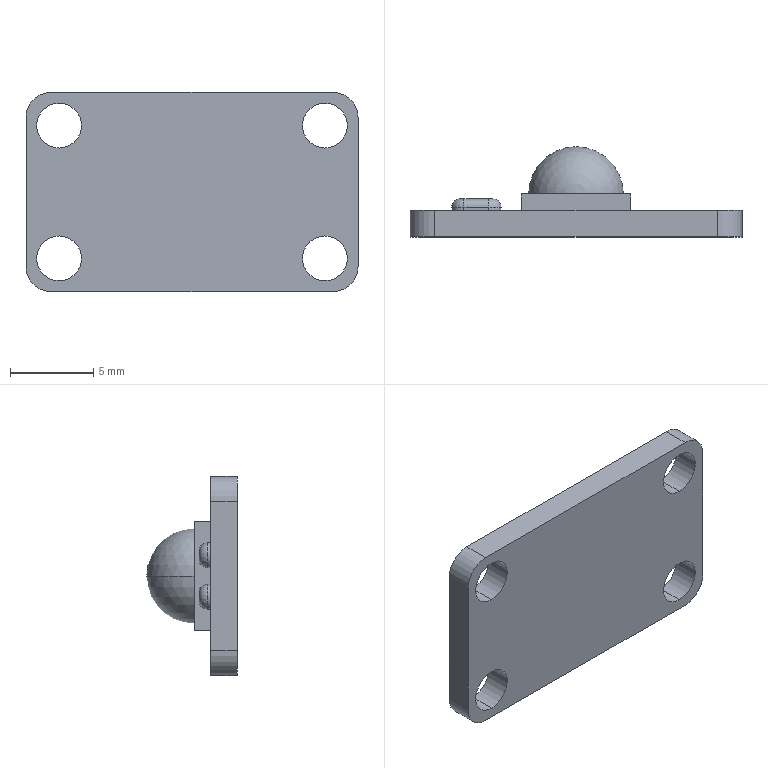Part | SolidWorks | features ICE 3, Fillet 2, Extrusion 1, Revolution 1 | 4 solids | 46 faces | box 20 x 5.45 x 12 mm | volume 441.181 mm3 | plane 20 | cylinder 20 | torus 4 | sphere 2 | commonest cylinder face diameters 2.7 x8 1 x4 1.5 x4 3 x4
STEP:
#1=CARTESIAN_POINT('',(0.,5.45,0.));
#2=VERTEX_POINT('',#1);
#3=CARTESIAN_POINT('',(2.85,2.6,0.));
#4=VERTEX_POINT('',#3);
#5=CARTESIAN_POINT('',(0.,2.6,0.));
#6=DIRECTION('',(0.,0.,-1.));
#7=DIRECTION('',(-1.,0.,0.));
#8=AXIS2_PLACEMENT_3D('',#5,#6,#7);
#9=CIRCLE('',#8,2.85);
#10=EDGE_CURVE('',#2,#4,#9,.T.);
#11=ORIENTED_EDGE('',*,*,#10,.F.);
#12=CARTESIAN_POINT('',(-2.85,2.6,0.));
#13=VERTEX_POINT('',#12);
#14=CARTESIAN_POINT('',(0.,2.6,0.));
#15=DIRECTION('',(0.,0.,1.));
#16=DIRECTION('',(1.,0.,0.));
#17=AXIS2_PLACEMENT_3D('',#14,#15,#16);
#18=CIRCLE('',#17,2.85);
#19=EDGE_CURVE('',#2,#13,#18,.T.);
#20=ORIENTED_EDGE('',*,*,#19,.T.);
#21=CARTESIAN_POINT('',(0.,2.6,0.));
#22=DIRECTION('',(0.,1.,0.));
#23=DIRECTION('',(0.,0.,1.));
#24=AXIS2_PLACEMENT_3D('',#21,#22,#23);
#25=CIRCLE('',#24,2.85);
#26=EDGE_CURVE('',#13,#4,#25,.T.);
#27=ORIENTED_EDGE('',*,*,#26,.T.);
#28=EDGE_LOOP('',(#11,#20,#27));
#29=FACE_OUTER_BOUND('',#28,.T.);
#30=CARTESIAN_POINT('',(0.,2.6,0.));
#31=DIRECTION('',(0.,0.,1.));
#32=DIRECTION('',(1.,0.,0.));
#33=AXIS2_PLACEMENT_3D('',#30,#31,#32);
#34=SPHERICAL_SURFACE('',#33,2.85);
#35=ADVANCED_FACE('',(#29),#34,.T.);
#36=CARTESIAN_POINT('',(3.3,1.6,3.3));
#37=VERTEX_POINT('',#36);
#38=CARTESIAN_POINT('',(3.3,1.6,-3.3));
#39=VERTEX_POINT('',#38);
#40=CARTESIAN_POINT('',(3.3,1.6,-3.3));
#41=DIRECTION('',(0.,0.,-1.));
#42=VECTOR('',#41,1000.);
#43=LINE('',#40,#42);
#44=EDGE_CURVE('',#37,#39,#43,.T.);
#45=ORIENTED_EDGE('',*,*,#44,.T.);
#46=CARTESIAN_POINT('',(3.3,2.6,-3.3));
#47=VERTEX_POINT('',#46);
#48=CARTESIAN_POINT('',(3.3,2.6,-3.3));
#49=DIRECTION('',(0.,-1.,0.));
#50=VECTOR('',#49,1000.);
#51=LINE('',#48,#50);
#52=EDGE_CURVE('',#47,#39,#51,.T.);
#53=ORIENTED_EDGE('',*,*,#52,.F.);
#54=CARTESIAN_POINT('',(3.3,2.6,3.3));
#55=VERTEX_POINT('',#54);
#56=CARTESIAN_POINT('',(3.3,2.6,-3.3));
#57=DIRECTION('',(0.,0.,-1.));
#58=VECTOR('',#57,1000.);
#59=LINE('',#56,#58);
#60=EDGE_CURVE('',#55,#47,#59,.T.);
#61=ORIENTED_EDGE('',*,*,#60,.F.);
#62=CARTESIAN_POINT('',(3.3,2.6,3.3));
#63=DIRECTION('',(0.,-1.,0.));
#64=VECTOR('',#63,1000.);
#65=LINE('',#62,#64);
#66=EDGE_CURVE('',#55,#37,#65,.T.);
#67=ORIENTED_EDGE('',*,*,#66,.T.);
#68=EDGE_LOOP('',(#45,#53,#61,#67));
#69=FACE_OUTER_BOUND('',#68,.T.);
#70=CARTESIAN_POINT('',(3.3,2.6,-3.3));
#71=DIRECTION('',(-1.,0.,0.));
#72=DIRECTION('',(0.,0.,1.));
#73=AXIS2_PLACEMENT_3D('',#70,#71,#72);
#74=PLANE('',#73);
#75=ADVANCED_FACE('',(#69),#74,.F.);
#76=CARTESIAN_POINT('',(-3.3,1.6,-3.3));
#77=VERTEX_POINT('',#76);
#78=CARTESIAN_POINT('',(-3.3,1.6,-3.3));
#79=DIRECTION('',(-1.,0.,0.));
#80=VECTOR('',#79,1000.);
#81=LINE('',#78,#80);
#82=EDGE_CURVE('',#39,#77,#81,.T.);
#83=ORIENTED_EDGE('',*,*,#82,.T.);
#84=CARTESIAN_POINT('',(-3.3,2.6,-3.3));
#85=VERTEX_POINT('',#84);
#86=CARTESIAN_POINT('',(-3.3,2.6,-3.3));
#87=DIRECTION('',(0.,-1.,0.));
#88=VECTOR('',#87,1000.);
#89=LINE('',#86,#88);
#90=EDGE_CURVE('',#85,#77,#89,.T.);
#91=ORIENTED_EDGE('',*,*,#90,.F.);
#92=CARTESIAN_POINT('',(-3.3,2.6,-3.3));
#93=DIRECTION('',(-1.,0.,0.));
#94=VECTOR('',#93,1000.);
#95=LINE('',#92,#94);
#96=EDGE_CURVE('',#47,#85,#95,.T.);
#97=ORIENTED_EDGE('',*,*,#96,.F.);
#98=ORIENTED_EDGE('',*,*,#52,.T.);
#99=EDGE_LOOP('',(#83,#91,#97,#98));
#100=FACE_OUTER_BOUND('',#99,.T.);
#101=CARTESIAN_POINT('',(-3.3,2.6,-3.3));
#102=DIRECTION('',(0.,0.,1.));
#103=DIRECTION('',(1.,0.,0.));
#104=AXIS2_PLACEMENT_3D('',#101,#102,#103);
#105=PLANE('',#104);
#106=ADVANCED_FACE('',(#100),#105,.F.);
#107=CARTESIAN_POINT('',(-3.3,1.6,3.3));
#108=VERTEX_POINT('',#107);
#109=CARTESIAN_POINT('',(-3.3,1.6,-3.3));
#110=DIRECTION('',(0.,0.,1.));
#111=VECTOR('',#110,1000.);
#112=LINE('',#109,#111);
#113=EDGE_CURVE('',#77,#108,#112,.T.);
#114=ORIENTED_EDGE('',*,*,#113,.T.);
#115=CARTESIAN_POINT('',(-3.3,2.6,3.3));
#116=VERTEX_POINT('',#115);
#117=CARTESIAN_POINT('',(-3.3,2.6,3.3));
#118=DIRECTION('',(0.,-1.,0.));
#119=VECTOR('',#118,1000.);
#120=LINE('',#117,#119);
#121=EDGE_CURVE('',#116,#108,#120,.T.);
#122=ORIENTED_EDGE('',*,*,#121,.F.);
#123=CARTESIAN_POINT('',(-3.3,2.6,-3.3));
#124=DIRECTION('',(0.,0.,1.));
#125=VECTOR('',#124,1000.);
#126=LINE('',#123,#125);
#127=EDGE_CURVE('',#85,#116,#126,.T.);
#128=ORIENTED_EDGE('',*,*,#127,.F.);
#129=ORIENTED_EDGE('',*,*,#90,.T.);
#130=EDGE_LOOP('',(#114,#122,#128,#129));
#131=FACE_OUTER_BOUND('',#130,.T.);
#132=CARTESIAN_POINT('',(-3.3,2.6,-3.3));
#133=DIRECTION('',(1.,0.,0.));
#134=DIRECTION('',(0.,0.,-1.));
#135=AXIS2_PLACEMENT_3D('',#132,#133,#134);
#136=PLANE('',#135);
#137=ADVANCED_FACE('',(#131),#136,.F.);
#138=CARTESIAN_POINT('',(-3.3,1.6,3.3));
#139=DIRECTION('',(1.,0.,0.));
#140=VECTOR('',#139,1000.);
#141=LINE('',#138,#140);
#142=EDGE_CURVE('',#108,#37,#141,.T.);
#143=ORIENTED_EDGE('',*,*,#142,.T.);
#144=ORIENTED_EDGE('',*,*,#66,.F.);
#145=CARTESIAN_POINT('',(-3.3,2.6,3.3));
#146=DIRECTION('',(1.,0.,0.));
#147=VECTOR('',#146,1000.);
#148=LINE('',#145,#147);
#149=EDGE_CURVE('',#116,#55,#148,.T.);
#150=ORIENTED_EDGE('',*,*,#149,.F.);
#151=ORIENTED_EDGE('',*,*,#121,.T.);
#152=EDGE_LOOP('',(#143,#144,#150,#151));
#153=FACE_OUTER_BOUND('',#152,.T.);
#154=CARTESIAN_POINT('',(-3.3,2.6,3.3));
#155=DIRECTION('',(0.,0.,-1.));
#156=DIRECTION('',(-1.,0.,0.));
#157=AXIS2_PLACEMENT_3D('',#154,#155,#156);
#158=PLANE('',#157);
#159=ADVANCED_FACE('',(#153),#158,.F.);
#160=CARTESIAN_POINT('',(0.,2.6,0.));
#161=DIRECTION('',(0.,1.,0.));
#162=DIRECTION('',(0.,0.,1.));
#163=AXIS2_PLACEMENT_3D('',#160,#161,#162);
#164=CIRCLE('',#163,2.85);
#165=EDGE_CURVE('',#4,#13,#164,.T.);
#166=ORIENTED_EDGE('',*,*,#165,.F.);
#167=ORIENTED_EDGE('',*,*,#26,.F.);
#168=EDGE_LOOP('',(#166,#167));
#169=FACE_BOUND('',#168,.T.);
#170=ORIENTED_EDGE('',*,*,#60,.T.);
#171=ORIENTED_EDGE('',*,*,#96,.T.);
#172=ORIENTED_EDGE('',*,*,#127,.T.);
#173=ORIENTED_EDGE('',*,*,#149,.T.);
#174=EDGE_LOOP('',(#170,#171,#172,#173));
#175=FACE_OUTER_BOUND('',#174,.T.);
#176=CARTESIAN_POINT('',(0.,2.6,0.));
#177=DIRECTION('',(0.,1.,0.));
#178=DIRECTION('',(0.,0.,1.));
#179=AXIS2_PLACEMENT_3D('',#176,#177,#178);
#180=PLANE('',#179);
#181=ADVANCED_FACE('',(#169,#175),#180,.T.);
#182=ORIENTED_EDGE('',*,*,#44,.F.);
#183=ORIENTED_EDGE('',*,*,#142,.F.);
#184=ORIENTED_EDGE('',*,*,#113,.F.);
#185=ORIENTED_EDGE('',*,*,#82,.F.);
#186=EDGE_LOOP('',(#182,#183,#184,#185));
#187=FACE_OUTER_BOUND('',#186,.T.);
#188=CARTESIAN_POINT('',(0.,1.6,0.));
#189=DIRECTION('',(0.,1.,0.));
#190=DIRECTION('',(0.,0.,1.));
#191=AXIS2_PLACEMENT_3D('',#188,#189,#190);
#192=PLANE('',#191);
#193=ADVANCED_FACE('',(#187),#192,.F.);
#194=ORIENTED_EDGE('',*,*,#19,.F.);
#195=ORIENTED_EDGE('',*,*,#10,.T.);
#196=ORIENTED_EDGE('',*,*,#165,.T.);
#197=EDGE_LOOP('',(#194,#195,#196));
#198=FACE_OUTER_BOUND('',#197,.T.);
#199=CARTESIAN_POINT('',(0.,2.6,0.));
#200=DIRECTION('',(0.,0.,1.));
#201=DIRECTION('',(1.,0.,0.));
#202=AXIS2_PLACEMENT_3D('',#199,#200,#201);
#203=SPHERICAL_SURFACE('',#202,2.85);
#204=ADVANCED_FACE('',(#198),#203,.T.);
#205=CLOSED_SHELL('',(#35,#75,#106,#137,#159,#181,#193,#204));
#206=MANIFOLD_SOLID_BREP('',#205);
#207=CARTESIAN_POINT('',(-8.,1.6,-5.35));
#208=VERTEX_POINT('',#207);
#209=CARTESIAN_POINT('',(-8.,1.6,-2.65));
#210=VERTEX_POINT('',#209);
#211=CARTESIAN_POINT('',(-8.,1.6,-4.));
#212=DIRECTION('',(0.,1.,0.));
#213=DIRECTION('',(0.,0.,1.));
#214=AXIS2_PLACEMENT_3D('',#211,#212,#213);
#215=CIRCLE('',#214,1.35);
#216=EDGE_CURVE('',#208,#210,#215,.T.);
#217=ORIENTED_EDGE('',*,*,#216,.T.);
#218=CARTESIAN_POINT('',(-8.,0.,-2.65));
#219=VERTEX_POINT('',#218);
#220=CARTESIAN_POINT('',(-8.,1.6,-2.65));
#221=DIRECTION('',(0.,-1.,0.));
#222=VECTOR('',#221,1000.);
#223=LINE('',#220,#222);
#224=EDGE_CURVE('',#210,#219,#223,.T.);
#225=ORIENTED_EDGE('',*,*,#224,.T.);
#226=CARTESIAN_POINT('',(-8.,0.,-5.35));
#227=VERTEX_POINT('',#226);
#228=CARTESIAN_POINT('',(-8.,0.,-4.));
#229=DIRECTION('',(0.,1.,0.));
#230=DIRECTION('',(0.,0.,1.));
#231=AXIS2_PLACEMENT_3D('',#228,#229,#230);
#232=CIRCLE('',#231,1.35);
#233=EDGE_CURVE('',#227,#219,#232,.T.);
#234=ORIENTED_EDGE('',*,*,#233,.F.);
#235=CARTESIAN_POINT('',(-8.,1.6,-5.35));
#236=DIRECTION('',(0.,-1.,0.));
#237=VECTOR('',#236,1000.);
#238=LINE('',#235,#237);
#239=EDGE_CURVE('',#208,#227,#238,.T.);
#240=ORIENTED_EDGE('',*,*,#239,.F.);
#241=EDGE_LOOP('',(#217,#225,#234,#240));
#242=FACE_OUTER_BOUND('',#241,.T.);
#243=CARTESIAN_POINT('',(-8.,1.6,-4.));
#244=DIRECTION('',(0.,-1.,0.));
#245=DIRECTION('',(0.,0.,-1.));
#246=AXIS2_PLACEMENT_3D('',#243,#244,#245);
#247=CYLINDRICAL_SURFACE('',#246,1.35);
#248=ADVANCED_FACE('',(#242),#247,.F.);
#249=CARTESIAN_POINT('',(8.,1.6,-5.35));
#250=VERTEX_POINT('',#249);
#251=CARTESIAN_POINT('',(8.,1.6,-2.65));
#252=VERTEX_POINT('',#251);
#253=CARTESIAN_POINT('',(8.,1.6,-4.));
#254=DIRECTION('',(0.,1.,0.));
#255=DIRECTION('',(0.,0.,1.));
#256=AXIS2_PLACEMENT_3D('',#253,#254,#255);
#257=CIRCLE('',#256,1.35);
#258=EDGE_CURVE('',#250,#252,#257,.T.);
#259=ORIENTED_EDGE('',*,*,#258,.T.);
#260=CARTESIAN_POINT('',(8.,0.,-2.65));
#261=VERTEX_POINT('',#260);
#262=CARTESIAN_POINT('',(8.,1.6,-2.65));
#263=DIRECTION('',(0.,-1.,0.));
#264=VECTOR('',#263,1000.);
#265=LINE('',#262,#264);
#266=EDGE_CURVE('',#252,#261,#265,.T.);
#267=ORIENTED_EDGE('',*,*,#266,.T.);
#268=CARTESIAN_POINT('',(8.,0.,-5.35));
#269=VERTEX_POINT('',#268);
#270=CARTESIAN_POINT('',(8.,0.,-4.));
#271=DIRECTION('',(0.,1.,0.));
#272=DIRECTION('',(0.,0.,1.));
#273=AXIS2_PLACEMENT_3D('',#270,#271,#272);
#274=CIRCLE('',#273,1.35);
#275=EDGE_CURVE('',#269,#261,#274,.T.);
#276=ORIENTED_EDGE('',*,*,#275,.F.);
#277=CARTESIAN_POINT('',(8.,1.6,-5.35));
#278=DIRECTION('',(0.,-1.,0.));
#279=VECTOR('',#278,1000.);
#280=LINE('',#277,#279);
#281=EDGE_CURVE('',#250,#269,#280,.T.);
#282=ORIENTED_EDGE('',*,*,#281,.F.);
#283=EDGE_LOOP('',(#259,#267,#276,#282));
#284=FACE_OUTER_BOUND('',#283,.T.);
#285=CARTESIAN_POINT('',(8.,1.6,-4.));
#286=DIRECTION('',(0.,-1.,0.));
#287=DIRECTION('',(0.,0.,-1.));
#288=AXIS2_PLACEMENT_3D('',#285,#286,#287);
#289=CYLINDRICAL_SURFACE('',#288,1.35);
#290=ADVANCED_FACE('',(#284),#289,.F.);
#291=CARTESIAN_POINT('',(8.,1.6,2.65));
#292=VERTEX_POINT('',#291);
#293=CARTESIAN_POINT('',(8.,1.6,5.35));
#294=VERTEX_POINT('',#293);
#295=CARTESIAN_POINT('',(8.,1.6,4.));
#296=DIRECTION('',(0.,1.,0.));
#297=DIRECTION('',(0.,0.,1.));
#298=AXIS2_PLACEMENT_3D('',#295,#296,#297);
#299=CIRCLE('',#298,1.35);
#300=EDGE_CURVE('',#292,#294,#299,.T.);
#301=ORIENTED_EDGE('',*,*,#300,.T.);
#302=CARTESIAN_POINT('',(8.,0.,5.35));
#303=VERTEX_POINT('',#302);
#304=CARTESIAN_POINT('',(8.,1.6,5.35));
#305=DIRECTION('',(0.,-1.,0.));
#306=VECTOR('',#305,1000.);
#307=LINE('',#304,#306);
#308=EDGE_CURVE('',#294,#303,#307,.T.);
#309=ORIENTED_EDGE('',*,*,#308,.T.);
#310=CARTESIAN_POINT('',(8.,0.,2.65));
#311=VERTEX_POINT('',#310);
#312=CARTESIAN_POINT('',(8.,0.,4.));
#313=DIRECTION('',(0.,1.,0.));
#314=DIRECTION('',(0.,0.,1.));
#315=AXIS2_PLACEMENT_3D('',#312,#313,#314);
#316=CIRCLE('',#315,1.35);
#317=EDGE_CURVE('',#311,#303,#316,.T.);
#318=ORIENTED_EDGE('',*,*,#317,.F.);
#319=CARTESIAN_POINT('',(8.,1.6,2.65));
#320=DIRECTION('',(0.,-1.,0.));
#321=VECTOR('',#320,1000.);
#322=LINE('',#319,#321);
#323=EDGE_CURVE('',#292,#311,#322,.T.);
#324=ORIENTED_EDGE('',*,*,#323,.F.);
#325=EDGE_LOOP('',(#301,#309,#318,#324));
#326=FACE_OUTER_BOUND('',#325,.T.);
#327=CARTESIAN_POINT('',(8.,1.6,4.));
#328=DIRECTION('',(0.,-1.,0.));
#329=DIRECTION('',(0.,0.,-1.));
#330=AXIS2_PLACEMENT_3D('',#327,#328,#329);
#331=CYLINDRICAL_SURFACE('',#330,1.35);
#332=ADVANCED_FACE('',(#326),#331,.F.);
#333=CARTESIAN_POINT('',(-8.,1.6,2.65));
#334=VERTEX_POINT('',#333);
#335=CARTESIAN_POINT('',(-8.,1.6,5.35));
#336=VERTEX_POINT('',#335);
#337=CARTESIAN_POINT('',(-8.,1.6,4.));
#338=DIRECTION('',(0.,1.,0.));
#339=DIRECTION('',(0.,0.,1.));
#340=AXIS2_PLACEMENT_3D('',#337,#338,#339);
#341=CIRCLE('',#340,1.35);
#342=EDGE_CURVE('',#334,#336,#341,.T.);
#343=ORIENTED_EDGE('',*,*,#342,.T.);
#344=CARTESIAN_POINT('',(-8.,0.,5.35));
#345=VERTEX_POINT('',#344);
#346=CARTESIAN_POINT('',(-8.,1.6,5.35));
#347=DIRECTION('',(0.,-1.,0.));
#348=VECTOR('',#347,1000.);
#349=LINE('',#346,#348);
#350=EDGE_CURVE('',#336,#345,#349,.T.);
#351=ORIENTED_EDGE('',*,*,#350,.T.);
#352=CARTESIAN_POINT('',(-8.,0.,2.65));
#353=VERTEX_POINT('',#352);
#354=CARTESIAN_POINT('',(-8.,0.,4.));
#355=DIRECTION('',(0.,1.,0.));
#356=DIRECTION('',(0.,0.,1.));
#357=AXIS2_PLACEMENT_3D('',#354,#355,#356);
#358=CIRCLE('',#357,1.35);
#359=EDGE_CURVE('',#353,#345,#358,.T.);
#360=ORIENTED_EDGE('',*,*,#359,.F.);
#361=CARTESIAN_POINT('',(-8.,1.6,2.65));
#362=DIRECTION('',(0.,-1.,0.));
#363=VECTOR('',#362,1000.);
#364=LINE('',#361,#363);
#365=EDGE_CURVE('',#334,#353,#364,.T.);
#366=ORIENTED_EDGE('',*,*,#365,.F.);
#367=EDGE_LOOP('',(#343,#351,#360,#366));
#368=FACE_OUTER_BOUND('',#367,.T.);
#369=CARTESIAN_POINT('',(-8.,1.6,4.));
#370=DIRECTION('',(0.,-1.,0.));
#371=DIRECTION('',(0.,0.,-1.));
#372=AXIS2_PLACEMENT_3D('',#369,#370,#371);
#373=CYLINDRICAL_SURFACE('',#372,1.35);
#374=ADVANCED_FACE('',(#368),#373,.F.);
#375=CARTESIAN_POINT('',(-10.,0.,4.5));
#376=VERTEX_POINT('',#375);
#377=CARTESIAN_POINT('',(-8.5,0.,6.));
#378=VERTEX_POINT('',#377);
#379=CARTESIAN_POINT('',(-8.5,0.,4.5));
#380=DIRECTION('',(0.,1.,0.));
#381=DIRECTION('',(0.,0.,-1.));
#382=AXIS2_PLACEMENT_3D('',#379,#380,#381);
#383=CIRCLE('',#382,1.5);
#384=EDGE_CURVE('',#376,#378,#383,.T.);
#385=ORIENTED_EDGE('',*,*,#384,.T.);
#386=CARTESIAN_POINT('',(-8.5,1.6,6.));
#387=VERTEX_POINT('',#386);
#388=CARTESIAN_POINT('',(-8.5,1.6,6.));
#389=DIRECTION('',(0.,-1.,0.));
#390=VECTOR('',#389,1000.);
#391=LINE('',#388,#390);
#392=EDGE_CURVE('',#387,#378,#391,.T.);
#393=ORIENTED_EDGE('',*,*,#392,.F.);
#394=CARTESIAN_POINT('',(-10.,1.6,4.5));
#395=VERTEX_POINT('',#394);
#396=CARTESIAN_POINT('',(-8.5,1.6,4.5));
#397=DIRECTION('',(0.,1.,0.));
#398=DIRECTION('',(0.,0.,-1.));
#399=AXIS2_PLACEMENT_3D('',#396,#397,#398);
#400=CIRCLE('',#399,1.5);
#401=EDGE_CURVE('',#395,#387,#400,.T.);
#402=ORIENTED_EDGE('',*,*,#401,.F.);
#403=CARTESIAN_POINT('',(-10.,1.6,4.5));
#404=DIRECTION('',(0.,-1.,0.));
#405=VECTOR('',#404,1000.);
#406=LINE('',#403,#405);
#407=EDGE_CURVE('',#395,#376,#406,.T.);
#408=ORIENTED_EDGE('',*,*,#407,.T.);
#409=EDGE_LOOP('',(#385,#393,#402,#408));
#410=FACE_OUTER_BOUND('',#409,.T.);
#411=CARTESIAN_POINT('',(-8.5,1.6,4.5));
#412=DIRECTION('',(0.,-1.,0.));
#413=DIRECTION('',(0.,0.,-1.));
#414=AXIS2_PLACEMENT_3D('',#411,#412,#413);
#415=CYLINDRICAL_SURFACE('',#414,1.5);
#416=ADVANCED_FACE('',(#410),#415,.T.);
#417=CARTESIAN_POINT('',(8.5,0.,6.));
#418=VERTEX_POINT('',#417);
#419=CARTESIAN_POINT('',(-8.5,0.,6.));
#420=DIRECTION('',(1.,0.,0.));
#421=VECTOR('',#420,1000.);
#422=LINE('',#419,#421);
#423=EDGE_CURVE('',#378,#418,#422,.T.);
#424=ORIENTED_EDGE('',*,*,#423,.T.);
#425=CARTESIAN_POINT('',(8.5,1.6,6.));
#426=VERTEX_POINT('',#425);
#427=CARTESIAN_POINT('',(8.5,1.6,6.));
#428=DIRECTION('',(0.,-1.,0.));
#429=VECTOR('',#428,1000.);
#430=LINE('',#427,#429);
#431=EDGE_CURVE('',#426,#418,#430,.T.);
#432=ORIENTED_EDGE('',*,*,#431,.F.);
#433=CARTESIAN_POINT('',(-8.5,1.6,6.));
#434=DIRECTION('',(1.,0.,0.));
#435=VECTOR('',#434,1000.);
#436=LINE('',#433,#435);
#437=EDGE_CURVE('',#387,#426,#436,.T.);
#438=ORIENTED_EDGE('',*,*,#437,.F.);
#439=ORIENTED_EDGE('',*,*,#392,.T.);
#440=EDGE_LOOP('',(#424,#432,#438,#439));
#441=FACE_OUTER_BOUND('',#440,.T.);
#442=CARTESIAN_POINT('',(-8.5,1.6,6.));
#443=DIRECTION('',(0.,0.,-1.));
#444=DIRECTION('',(-1.,0.,0.));
#445=AXIS2_PLACEMENT_3D('',#442,#443,#444);
#446=PLANE('',#445);
#447=ADVANCED_FACE('',(#441),#446,.F.);
#448=CARTESIAN_POINT('',(10.,0.,4.5));
#449=VERTEX_POINT('',#448);
#450=CARTESIAN_POINT('',(8.5,0.,4.5));
#451=DIRECTION('',(0.,1.,0.));
#452=DIRECTION('',(0.,0.,1.));
#453=AXIS2_PLACEMENT_3D('',#450,#451,#452);
#454=CIRCLE('',#453,1.5);
#455=EDGE_CURVE('',#418,#449,#454,.T.);
#456=ORIENTED_EDGE('',*,*,#455,.T.);
#457=CARTESIAN_POINT('',(10.,1.6,4.5));
#458=VERTEX_POINT('',#457);
#459=CARTESIAN_POINT('',(10.,1.6,4.5));
#460=DIRECTION('',(0.,-1.,0.));
#461=VECTOR('',#460,1000.);
#462=LINE('',#459,#461);
#463=EDGE_CURVE('',#458,#449,#462,.T.);
#464=ORIENTED_EDGE('',*,*,#463,.F.);
#465=CARTESIAN_POINT('',(8.5,1.6,4.5));
#466=DIRECTION('',(0.,1.,0.));
#467=DIRECTION('',(0.,0.,1.));
#468=AXIS2_PLACEMENT_3D('',#465,#466,#467);
#469=CIRCLE('',#468,1.5);
#470=EDGE_CURVE('',#426,#458,#469,.T.);
#471=ORIENTED_EDGE('',*,*,#470,.F.);
#472=ORIENTED_EDGE('',*,*,#431,.T.);
#473=EDGE_LOOP('',(#456,#464,#471,#472));
#474=FACE_OUTER_BOUND('',#473,.T.);
#475=CARTESIAN_POINT('',(8.5,1.6,4.5));
#476=DIRECTION('',(0.,-1.,0.));
#477=DIRECTION('',(0.,0.,-1.));
#478=AXIS2_PLACEMENT_3D('',#475,#476,#477);
#479=CYLINDRICAL_SURFACE('',#478,1.5);
#480=ADVANCED_FACE('',(#474),#479,.T.);
#481=CARTESIAN_POINT('',(10.,0.,-4.5));
#482=VERTEX_POINT('',#481);
#483=CARTESIAN_POINT('',(10.,0.,4.5));
#484=DIRECTION('',(0.,0.,-1.));
#485=VECTOR('',#484,1000.);
#486=LINE('',#483,#485);
#487=EDGE_CURVE('',#449,#482,#486,.T.);
#488=ORIENTED_EDGE('',*,*,#487,.T.);
#489=CARTESIAN_POINT('',(10.,1.6,-4.5));
#490=VERTEX_POINT('',#489);
#491=CARTESIAN_POINT('',(10.,1.6,-4.5));
#492=DIRECTION('',(0.,-1.,0.));
#493=VECTOR('',#492,1000.);
#494=LINE('',#491,#493);
#495=EDGE_CURVE('',#490,#482,#494,.T.);
#496=ORIENTED_EDGE('',*,*,#495,.F.);
#497=CARTESIAN_POINT('',(10.,1.6,4.5));
#498=DIRECTION('',(0.,0.,-1.));
#499=VECTOR('',#498,1000.);
#500=LINE('',#497,#499);
#501=EDGE_CURVE('',#458,#490,#500,.T.);
#502=ORIENTED_EDGE('',*,*,#501,.F.);
#503=ORIENTED_EDGE('',*,*,#463,.T.);
#504=EDGE_LOOP('',(#488,#496,#502,#503));
#505=FACE_OUTER_BOUND('',#504,.T.);
#506=CARTESIAN_POINT('',(10.,1.6,4.5));
#507=DIRECTION('',(-1.,0.,0.));
#508=DIRECTION('',(0.,0.,1.));
#509=AXIS2_PLACEMENT_3D('',#506,#507,#508);
#510=PLANE('',#509);
#511=ADVANCED_FACE('',(#505),#510,.F.);
#512=CARTESIAN_POINT('',(8.5,0.,-6.));
#513=VERTEX_POINT('',#512);
#514=CARTESIAN_POINT('',(8.5,0.,-4.5));
#515=DIRECTION('',(0.,1.,0.));
#516=DIRECTION('',(0.,0.,-1.));
#517=AXIS2_PLACEMENT_3D('',#514,#515,#516);
#518=CIRCLE('',#517,1.5);
#519=EDGE_CURVE('',#482,#513,#518,.T.);
#520=ORIENTED_EDGE('',*,*,#519,.T.);
#521=CARTESIAN_POINT('',(8.5,1.6,-6.));
#522=VERTEX_POINT('',#521);
#523=CARTESIAN_POINT('',(8.5,1.6,-6.));
#524=DIRECTION('',(0.,-1.,0.));
#525=VECTOR('',#524,1000.);
#526=LINE('',#523,#525);
#527=EDGE_CURVE('',#522,#513,#526,.T.);
#528=ORIENTED_EDGE('',*,*,#527,.F.);
#529=CARTESIAN_POINT('',(8.5,1.6,-4.5));
#530=DIRECTION('',(0.,1.,0.));
#531=DIRECTION('',(0.,0.,-1.));
#532=AXIS2_PLACEMENT_3D('',#529,#530,#531);
#533=CIRCLE('',#532,1.5);
#534=EDGE_CURVE('',#490,#522,#533,.T.);
#535=ORIENTED_EDGE('',*,*,#534,.F.);
#536=ORIENTED_EDGE('',*,*,#495,.T.);
#537=EDGE_LOOP('',(#520,#528,#535,#536));
#538=FACE_OUTER_BOUND('',#537,.T.);
#539=CARTESIAN_POINT('',(8.5,1.6,-4.5));
#540=DIRECTION('',(0.,-1.,0.));
#541=DIRECTION('',(0.,0.,-1.));
#542=AXIS2_PLACEMENT_3D('',#539,#540,#541);
#543=CYLINDRICAL_SURFACE('',#542,1.5);
#544=ADVANCED_FACE('',(#538),#543,.T.);
#545=CARTESIAN_POINT('',(-8.5,0.,-6.));
#546=VERTEX_POINT('',#545);
#547=CARTESIAN_POINT('',(-8.5,0.,-6.));
#548=DIRECTION('',(-1.,0.,0.));
#549=VECTOR('',#548,1000.);
#550=LINE('',#547,#549);
#551=EDGE_CURVE('',#513,#546,#550,.T.);
#552=ORIENTED_EDGE('',*,*,#551,.T.);
#553=CARTESIAN_POINT('',(-8.5,1.6,-6.));
#554=VERTEX_POINT('',#553);
#555=CARTESIAN_POINT('',(-8.5,1.6,-6.));
#556=DIRECTION('',(0.,-1.,0.));
#557=VECTOR('',#556,1000.);
#558=LINE('',#555,#557);
#559=EDGE_CURVE('',#554,#546,#558,.T.);
#560=ORIENTED_EDGE('',*,*,#559,.F.);
#561=CARTESIAN_POINT('',(-8.5,1.6,-6.));
#562=DIRECTION('',(-1.,0.,0.));
#563=VECTOR('',#562,1000.);
#564=LINE('',#561,#563);
#565=EDGE_CURVE('',#522,#554,#564,.T.);
#566=ORIENTED_EDGE('',*,*,#565,.F.);
#567=ORIENTED_EDGE('',*,*,#527,.T.);
#568=EDGE_LOOP('',(#552,#560,#566,#567));
#569=FACE_OUTER_BOUND('',#568,.T.);
#570=CARTESIAN_POINT('',(-8.5,1.6,-6.));
#571=DIRECTION('',(0.,0.,1.));
#572=DIRECTION('',(1.,0.,0.));
#573=AXIS2_PLACEMENT_3D('',#570,#571,#572);
#574=PLANE('',#573);
#575=ADVANCED_FACE('',(#569),#574,.F.);
#576=CARTESIAN_POINT('',(-10.,0.,-4.5));
#577=VERTEX_POINT('',#576);
#578=CARTESIAN_POINT('',(-8.5,0.,-4.5));
#579=DIRECTION('',(0.,1.,0.));
#580=DIRECTION('',(0.,0.,-1.));
#581=AXIS2_PLACEMENT_3D('',#578,#579,#580);
#582=CIRCLE('',#581,1.5);
#583=EDGE_CURVE('',#546,#577,#582,.T.);
#584=ORIENTED_EDGE('',*,*,#583,.T.);
#585=CARTESIAN_POINT('',(-10.,1.6,-4.5));
#586=VERTEX_POINT('',#585);
#587=CARTESIAN_POINT('',(-10.,1.6,-4.5));
#588=DIRECTION('',(0.,-1.,0.));
#589=VECTOR('',#588,1000.);
#590=LINE('',#587,#589);
#591=EDGE_CURVE('',#586,#577,#590,.T.);
#592=ORIENTED_EDGE('',*,*,#591,.F.);
#593=CARTESIAN_POINT('',(-8.5,1.6,-4.5));
#594=DIRECTION('',(0.,1.,0.));
#595=DIRECTION('',(0.,0.,-1.));
#596=AXIS2_PLACEMENT_3D('',#593,#594,#595);
#597=CIRCLE('',#596,1.5);
#598=EDGE_CURVE('',#554,#586,#597,.T.);
#599=ORIENTED_EDGE('',*,*,#598,.F.);
#600=ORIENTED_EDGE('',*,*,#559,.T.);
#601=EDGE_LOOP('',(#584,#592,#599,#600));
#602=FACE_OUTER_BOUND('',#601,.T.);
#603=CARTESIAN_POINT('',(-8.5,1.6,-4.5));
#604=DIRECTION('',(0.,-1.,0.));
#605=DIRECTION('',(0.,0.,-1.));
#606=AXIS2_PLACEMENT_3D('',#603,#604,#605);
#607=CYLINDRICAL_SURFACE('',#606,1.5);
#608=ADVANCED_FACE('',(#602),#607,.T.);
#609=CARTESIAN_POINT('',(-10.,0.,4.5));
#610=DIRECTION('',(0.,0.,1.));
#611=VECTOR('',#610,1000.);
#612=LINE('',#609,#611);
#613=EDGE_CURVE('',#577,#376,#612,.T.);
#614=ORIENTED_EDGE('',*,*,#613,.T.);
#615=ORIENTED_EDGE('',*,*,#407,.F.);
#616=CARTESIAN_POINT('',(-10.,1.6,4.5));
#617=DIRECTION('',(0.,0.,1.));
#618=VECTOR('',#617,1000.);
#619=LINE('',#616,#618);
#620=EDGE_CURVE('',#586,#395,#619,.T.);
#621=ORIENTED_EDGE('',*,*,#620,.F.);
#622=ORIENTED_EDGE('',*,*,#591,.T.);
#623=EDGE_LOOP('',(#614,#615,#621,#622));
#624=FACE_OUTER_BOUND('',#623,.T.);
#625=CARTESIAN_POINT('',(-10.,1.6,4.5));
#626=DIRECTION('',(1.,0.,0.));
#627=DIRECTION('',(0.,0.,-1.));
#628=AXIS2_PLACEMENT_3D('',#625,#626,#627);
#629=PLANE('',#628);
#630=ADVANCED_FACE('',(#624),#629,.F.);
#631=ORIENTED_EDGE('',*,*,#216,.F.);
#632=CARTESIAN_POINT('',(-8.,1.6,-4.));
#633=DIRECTION('',(0.,1.,0.));
#634=DIRECTION('',(0.,0.,1.));
#635=AXIS2_PLACEMENT_3D('',#632,#633,#634);
#636=CIRCLE('',#635,1.35);
#637=EDGE_CURVE('',#210,#208,#636,.T.);
#638=ORIENTED_EDGE('',*,*,#637,.F.);
#639=EDGE_LOOP('',(#631,#638));
#640=FACE_BOUND('',#639,.T.);
#641=ORIENTED_EDGE('',*,*,#258,.F.);
#642=CARTESIAN_POINT('',(8.,1.6,-4.));
#643=DIRECTION('',(0.,1.,0.));
#644=DIRECTION('',(0.,0.,1.));
#645=AXIS2_PLACEMENT_3D('',#642,#643,#644);
#646=CIRCLE('',#645,1.35);
#647=EDGE_CURVE('',#252,#250,#646,.T.);
#648=ORIENTED_EDGE('',*,*,#647,.F.);
#649=EDGE_LOOP('',(#641,#648));
#650=FACE_BOUND('',#649,.T.);
#651=ORIENTED_EDGE('',*,*,#300,.F.);
#652=CARTESIAN_POINT('',(8.,1.6,4.));
#653=DIRECTION('',(0.,1.,0.));
#654=DIRECTION('',(0.,0.,1.));
#655=AXIS2_PLACEMENT_3D('',#652,#653,#654);
#656=CIRCLE('',#655,1.35);
#657=EDGE_CURVE('',#294,#292,#656,.T.);
#658=ORIENTED_EDGE('',*,*,#657,.F.);
#659=EDGE_LOOP('',(#651,#658));
#660=FACE_BOUND('',#659,.T.);
#661=ORIENTED_EDGE('',*,*,#342,.F.);
#662=CARTESIAN_POINT('',(-8.,1.6,4.));
#663=DIRECTION('',(0.,1.,0.));
#664=DIRECTION('',(0.,0.,1.));
#665=AXIS2_PLACEMENT_3D('',#662,#663,#664);
#666=CIRCLE('',#665,1.35);
#667=EDGE_CURVE('',#336,#334,#666,.T.);
#668=ORIENTED_EDGE('',*,*,#667,.F.);
#669=EDGE_LOOP('',(#661,#668));
#670=FACE_BOUND('',#669,.T.);
#671=ORIENTED_EDGE('',*,*,#401,.T.);
#672=ORIENTED_EDGE('',*,*,#437,.T.);
#673=ORIENTED_EDGE('',*,*,#470,.T.);
#674=ORIENTED_EDGE('',*,*,#501,.T.);
#675=ORIENTED_EDGE('',*,*,#534,.T.);
#676=ORIENTED_EDGE('',*,*,#565,.T.);
#677=ORIENTED_EDGE('',*,*,#598,.T.);
#678=ORIENTED_EDGE('',*,*,#620,.T.);
#679=EDGE_LOOP('',(#671,#672,#673,#674,#675,#676,#677,#678));
#680=FACE_OUTER_BOUND('',#679,.T.);
#681=CARTESIAN_POINT('',(-8.5,1.6,4.5));
#682=DIRECTION('',(0.,-1.,0.));
#683=DIRECTION('',(0.,0.,-1.));
#684=AXIS2_PLACEMENT_3D('',#681,#682,#683);
#685=PLANE('',#684);
#686=ADVANCED_FACE('',(#640,#650,#660,#670,#680),#685,.F.);
#687=ORIENTED_EDGE('',*,*,#233,.T.);
#688=CARTESIAN_POINT('',(-8.,0.,-4.));
#689=DIRECTION('',(0.,1.,0.));
#690=DIRECTION('',(0.,0.,1.));
#691=AXIS2_PLACEMENT_3D('',#688,#689,#690);
#692=CIRCLE('',#691,1.35);
#693=EDGE_CURVE('',#219,#227,#692,.T.);
#694=ORIENTED_EDGE('',*,*,#693,.T.);
#695=EDGE_LOOP('',(#687,#694));
#696=FACE_BOUND('',#695,.T.);
#697=ORIENTED_EDGE('',*,*,#275,.T.);
#698=CARTESIAN_POINT('',(8.,0.,-4.));
#699=DIRECTION('',(0.,1.,0.));
#700=DIRECTION('',(0.,0.,1.));
#701=AXIS2_PLACEMENT_3D('',#698,#699,#700);
#702=CIRCLE('',#701,1.35);
#703=EDGE_CURVE('',#261,#269,#702,.T.);
#704=ORIENTED_EDGE('',*,*,#703,.T.);
#705=EDGE_LOOP('',(#697,#704));
#706=FACE_BOUND('',#705,.T.);
#707=ORIENTED_EDGE('',*,*,#317,.T.);
#708=CARTESIAN_POINT('',(8.,0.,4.));
#709=DIRECTION('',(0.,1.,0.));
#710=DIRECTION('',(0.,0.,1.));
#711=AXIS2_PLACEMENT_3D('',#708,#709,#710);
#712=CIRCLE('',#711,1.35);
#713=EDGE_CURVE('',#303,#311,#712,.T.);
#714=ORIENTED_EDGE('',*,*,#713,.T.);
#715=EDGE_LOOP('',(#707,#714));
#716=FACE_BOUND('',#715,.T.);
#717=ORIENTED_EDGE('',*,*,#359,.T.);
#718=CARTESIAN_POINT('',(-8.,0.,4.));
#719=DIRECTION('',(0.,1.,0.));
#720=DIRECTION('',(0.,0.,1.));
#721=AXIS2_PLACEMENT_3D('',#718,#719,#720);
#722=CIRCLE('',#721,1.35);
#723=EDGE_CURVE('',#345,#353,#722,.T.);
#724=ORIENTED_EDGE('',*,*,#723,.T.);
#725=EDGE_LOOP('',(#717,#724));
#726=FACE_BOUND('',#725,.T.);
#727=ORIENTED_EDGE('',*,*,#384,.F.);
#728=ORIENTED_EDGE('',*,*,#613,.F.);
#729=ORIENTED_EDGE('',*,*,#583,.F.);
#730=ORIENTED_EDGE('',*,*,#551,.F.);
#731=ORIENTED_EDGE('',*,*,#519,.F.);
#732=ORIENTED_EDGE('',*,*,#487,.F.);
#733=ORIENTED_EDGE('',*,*,#455,.F.);
#734=ORIENTED_EDGE('',*,*,#423,.F.);
#735=EDGE_LOOP('',(#727,#728,#729,#730,#731,#732,#733,#734));
#736=FACE_OUTER_BOUND('',#735,.T.);
#737=CARTESIAN_POINT('',(-8.5,0.,4.5));
#738=DIRECTION('',(0.,-1.,0.));
#739=DIRECTION('',(0.,0.,-1.));
#740=AXIS2_PLACEMENT_3D('',#737,#738,#739);
#741=PLANE('',#740);
#742=ADVANCED_FACE('',(#696,#706,#716,#726,#736),#741,.T.);
#743=ORIENTED_EDGE('',*,*,#350,.F.);
#744=ORIENTED_EDGE('',*,*,#667,.T.);
#745=ORIENTED_EDGE('',*,*,#365,.T.);
#746=ORIENTED_EDGE('',*,*,#723,.F.);
#747=EDGE_LOOP('',(#743,#744,#745,#746));
#748=FACE_OUTER_BOUND('',#747,.T.);
#749=CARTESIAN_POINT('',(-8.,1.6,4.));
#750=DIRECTION('',(0.,-1.,0.));
#751=DIRECTION('',(0.,0.,-1.));
#752=AXIS2_PLACEMENT_3D('',#749,#750,#751);
#753=CYLINDRICAL_SURFACE('',#752,1.35);
#754=ADVANCED_FACE('',(#748),#753,.F.);
#755=ORIENTED_EDGE('',*,*,#308,.F.);
#756=ORIENTED_EDGE('',*,*,#657,.T.);
#757=ORIENTED_EDGE('',*,*,#323,.T.);
#758=ORIENTED_EDGE('',*,*,#713,.F.);
#759=EDGE_LOOP('',(#755,#756,#757,#758));
#760=FACE_OUTER_BOUND('',#759,.T.);
#761=CARTESIAN_POINT('',(8.,1.6,4.));
#762=DIRECTION('',(0.,-1.,0.));
#763=DIRECTION('',(0.,0.,-1.));
#764=AXIS2_PLACEMENT_3D('',#761,#762,#763);
#765=CYLINDRICAL_SURFACE('',#764,1.35);
#766=ADVANCED_FACE('',(#760),#765,.F.);
#767=ORIENTED_EDGE('',*,*,#266,.F.);
#768=ORIENTED_EDGE('',*,*,#647,.T.);
#769=ORIENTED_EDGE('',*,*,#281,.T.);
#770=ORIENTED_EDGE('',*,*,#703,.F.);
#771=EDGE_LOOP('',(#767,#768,#769,#770));
#772=FACE_OUTER_BOUND('',#771,.T.);
#773=CARTESIAN_POINT('',(8.,1.6,-4.));
#774=DIRECTION('',(0.,-1.,0.));
#775=DIRECTION('',(0.,0.,-1.));
#776=AXIS2_PLACEMENT_3D('',#773,#774,#775);
#777=CYLINDRICAL_SURFACE('',#776,1.35);
#778=ADVANCED_FACE('',(#772),#777,.F.);
#779=ORIENTED_EDGE('',*,*,#224,.F.);
#780=ORIENTED_EDGE('',*,*,#637,.T.);
#781=ORIENTED_EDGE('',*,*,#239,.T.);
#782=ORIENTED_EDGE('',*,*,#693,.F.);
#783=EDGE_LOOP('',(#779,#780,#781,#782));
#784=FACE_OUTER_BOUND('',#783,.T.);
#785=CARTESIAN_POINT('',(-8.,1.6,-4.));
#786=DIRECTION('',(0.,-1.,0.));
#787=DIRECTION('',(0.,0.,-1.));
#788=AXIS2_PLACEMENT_3D('',#785,#786,#787);
#789=CYLINDRICAL_SURFACE('',#788,1.35);
#790=ADVANCED_FACE('',(#784),#789,.F.);
#791=CLOSED_SHELL('',(#248,#290,#332,#374,#416,#447,#480,#511,#544,#575,#608,#630,#686,#742,#754,#766,#778,#790));
#792=MANIFOLD_SOLID_BREP('',#791);
#793=CARTESIAN_POINT('',(-6.75,1.8,-0.5));
#794=VERTEX_POINT('',#793);
#795=CARTESIAN_POINT('',(-6.75,1.6,-0.5));
#796=VERTEX_POINT('',#795);
#797=CARTESIAN_POINT('',(-6.75,2.3,-0.5));
#798=DIRECTION('',(0.,-1.,0.));
#799=VECTOR('',#798,1000.);
#800=LINE('',#797,#799);
#801=EDGE_CURVE('',#794,#796,#800,.T.);
#802=ORIENTED_EDGE('',*,*,#801,.F.);
#803=CARTESIAN_POINT('',(-6.75,1.8,-2.));
#804=VERTEX_POINT('',#803);
#805=CARTESIAN_POINT('',(-6.75,1.8,-1.25));
#806=DIRECTION('',(0.,-1.,0.));
#807=DIRECTION('',(0.,0.,1.));
#808=AXIS2_PLACEMENT_3D('',#805,#806,#807);
#809=CIRCLE('',#808,0.75);
#810=EDGE_CURVE('',#794,#804,#809,.T.);
#811=ORIENTED_EDGE('',*,*,#810,.T.);
#812=CARTESIAN_POINT('',(-6.75,1.6,-2.));
#813=VERTEX_POINT('',#812);
#814=CARTESIAN_POINT('',(-6.75,2.3,-2.));
#815=DIRECTION('',(0.,-1.,0.));
#816=VECTOR('',#815,1000.);
#817=LINE('',#814,#816);
#818=EDGE_CURVE('',#804,#813,#817,.T.);
#819=ORIENTED_EDGE('',*,*,#818,.T.);
#820=CARTESIAN_POINT('',(-6.75,1.6,-1.25));
#821=DIRECTION('',(0.,1.,0.));
#822=DIRECTION('',(0.,0.,1.));
#823=AXIS2_PLACEMENT_3D('',#820,#821,#822);
#824=CIRCLE('',#823,0.75);
#825=EDGE_CURVE('',#813,#796,#824,.T.);
#826=ORIENTED_EDGE('',*,*,#825,.T.);
#827=EDGE_LOOP('',(#802,#811,#819,#826));
#828=FACE_OUTER_BOUND('',#827,.T.);
#829=CARTESIAN_POINT('',(-6.75,2.3,-1.25));
#830=DIRECTION('',(0.,-1.,0.));
#831=DIRECTION('',(0.,0.,-1.));
#832=AXIS2_PLACEMENT_3D('',#829,#830,#831);
#833=CYLINDRICAL_SURFACE('',#832,0.75);
#834=ADVANCED_FACE('',(#828),#833,.T.);
#835=CARTESIAN_POINT('',(-5.25,1.8,-0.5));
#836=VERTEX_POINT('',#835);
#837=CARTESIAN_POINT('',(-5.25,1.6,-0.5));
#838=VERTEX_POINT('',#837);
#839=CARTESIAN_POINT('',(-5.25,2.3,-0.5));
#840=DIRECTION('',(0.,-1.,0.));
#841=VECTOR('',#840,1000.);
#842=LINE('',#839,#841);
#843=EDGE_CURVE('',#836,#838,#842,.T.);
#844=ORIENTED_EDGE('',*,*,#843,.F.);
#845=CARTESIAN_POINT('',(-6.75,1.8,-0.5));
#846=DIRECTION('',(-1.,0.,0.));
#847=VECTOR('',#846,1000.);
#848=LINE('',#845,#847);
#849=EDGE_CURVE('',#836,#794,#848,.T.);
#850=ORIENTED_EDGE('',*,*,#849,.T.);
#851=ORIENTED_EDGE('',*,*,#801,.T.);
#852=CARTESIAN_POINT('',(-6.75,1.6,-0.5));
#853=DIRECTION('',(1.,0.,0.));
#854=VECTOR('',#853,1000.);
#855=LINE('',#852,#854);
#856=EDGE_CURVE('',#796,#838,#855,.T.);
#857=ORIENTED_EDGE('',*,*,#856,.T.);
#858=EDGE_LOOP('',(#844,#850,#851,#857));
#859=FACE_OUTER_BOUND('',#858,.T.);
#860=CARTESIAN_POINT('',(-6.75,2.3,-0.5));
#861=DIRECTION('',(0.,0.,-1.));
#862=DIRECTION('',(-1.,0.,0.));
#863=AXIS2_PLACEMENT_3D('',#860,#861,#862);
#864=PLANE('',#863);
#865=ADVANCED_FACE('',(#859),#864,.F.);
#866=CARTESIAN_POINT('',(-5.25,1.8,-2.));
#867=VERTEX_POINT('',#866);
#868=CARTESIAN_POINT('',(-5.25,1.6,-2.));
#869=VERTEX_POINT('',#868);
#870=CARTESIAN_POINT('',(-5.25,2.3,-2.));
#871=DIRECTION('',(0.,-1.,0.));
#872=VECTOR('',#871,1000.);
#873=LINE('',#870,#872);
#874=EDGE_CURVE('',#867,#869,#873,.T.);
#875=ORIENTED_EDGE('',*,*,#874,.F.);
#876=CARTESIAN_POINT('',(-5.25,1.8,-1.25));
#877=DIRECTION('',(0.,-1.,0.));
#878=DIRECTION('',(0.,0.,1.));
#879=AXIS2_PLACEMENT_3D('',#876,#877,#878);
#880=CIRCLE('',#879,0.75);
#881=EDGE_CURVE('',#867,#836,#880,.T.);
#882=ORIENTED_EDGE('',*,*,#881,.T.);
#883=ORIENTED_EDGE('',*,*,#843,.T.);
#884=CARTESIAN_POINT('',(-5.25,1.6,-1.25));
#885=DIRECTION('',(0.,1.,0.));
#886=DIRECTION('',(0.,0.,1.));
#887=AXIS2_PLACEMENT_3D('',#884,#885,#886);
#888=CIRCLE('',#887,0.75);
#889=EDGE_CURVE('',#838,#869,#888,.T.);
#890=ORIENTED_EDGE('',*,*,#889,.T.);
#891=EDGE_LOOP('',(#875,#882,#883,#890));
#892=FACE_OUTER_BOUND('',#891,.T.);
#893=CARTESIAN_POINT('',(-5.25,2.3,-1.25));
#894=DIRECTION('',(0.,-1.,0.));
#895=DIRECTION('',(0.,0.,-1.));
#896=AXIS2_PLACEMENT_3D('',#893,#894,#895);
#897=CYLINDRICAL_SURFACE('',#896,0.75);
#898=ADVANCED_FACE('',(#892),#897,.T.);
#899=ORIENTED_EDGE('',*,*,#818,.F.);
#900=CARTESIAN_POINT('',(-5.25,1.8,-2.));
#901=DIRECTION('',(1.,0.,0.));
#902=VECTOR('',#901,1000.);
#903=LINE('',#900,#902);
#904=EDGE_CURVE('',#804,#867,#903,.T.);
#905=ORIENTED_EDGE('',*,*,#904,.T.);
#906=ORIENTED_EDGE('',*,*,#874,.T.);
#907=CARTESIAN_POINT('',(-6.75,1.6,-2.));
#908=DIRECTION('',(-1.,0.,0.));
#909=VECTOR('',#908,1000.);
#910=LINE('',#907,#909);
#911=EDGE_CURVE('',#869,#813,#910,.T.);
#912=ORIENTED_EDGE('',*,*,#911,.T.);
#913=EDGE_LOOP('',(#899,#905,#906,#912));
#914=FACE_OUTER_BOUND('',#913,.T.);
#915=CARTESIAN_POINT('',(-6.75,2.3,-2.));
#916=DIRECTION('',(0.,0.,1.));
#917=DIRECTION('',(1.,0.,0.));
#918=AXIS2_PLACEMENT_3D('',#915,#916,#917);
#919=PLANE('',#918);
#920=ADVANCED_FACE('',(#914),#919,.F.);
#921=CARTESIAN_POINT('',(-5.25,2.3,-1.));
#922=VERTEX_POINT('',#921);
#923=CARTESIAN_POINT('',(-5.25,2.3,-1.5));
#924=VERTEX_POINT('',#923);
#925=CARTESIAN_POINT('',(-5.25,2.3,-1.25));
#926=DIRECTION('',(0.,1.,0.));
#927=DIRECTION('',(0.,0.,1.));
#928=AXIS2_PLACEMENT_3D('',#925,#926,#927);
#929=CIRCLE('',#928,0.25);
#930=EDGE_CURVE('',#922,#924,#929,.T.);
#931=ORIENTED_EDGE('',*,*,#930,.T.);
#932=CARTESIAN_POINT('',(-6.75,2.3,-1.5));
#933=VERTEX_POINT('',#932);
#934=CARTESIAN_POINT('',(-6.75,2.3,-1.5));
#935=DIRECTION('',(-1.,0.,0.));
#936=VECTOR('',#935,1000.);
#937=LINE('',#934,#936);
#938=EDGE_CURVE('',#924,#933,#937,.T.);
#939=ORIENTED_EDGE('',*,*,#938,.T.);
#940=CARTESIAN_POINT('',(-6.75,2.3,-1.));
#941=VERTEX_POINT('',#940);
#942=CARTESIAN_POINT('',(-6.75,2.3,-1.25));
#943=DIRECTION('',(0.,1.,0.));
#944=DIRECTION('',(0.,0.,1.));
#945=AXIS2_PLACEMENT_3D('',#942,#943,#944);
#946=CIRCLE('',#945,0.25);
#947=EDGE_CURVE('',#933,#941,#946,.T.);
#948=ORIENTED_EDGE('',*,*,#947,.T.);
#949=CARTESIAN_POINT('',(-5.25,2.3,-1.));
#950=DIRECTION('',(1.,0.,0.));
#951=VECTOR('',#950,1000.);
#952=LINE('',#949,#951);
#953=EDGE_CURVE('',#941,#922,#952,.T.);
#954=ORIENTED_EDGE('',*,*,#953,.T.);
#955=EDGE_LOOP('',(#931,#939,#948,#954));
#956=FACE_OUTER_BOUND('',#955,.T.);
#957=CARTESIAN_POINT('',(-6.75,2.3,-1.25));
#958=DIRECTION('',(0.,1.,0.));
#959=DIRECTION('',(0.,0.,1.));
#960=AXIS2_PLACEMENT_3D('',#957,#958,#959);
#961=PLANE('',#960);
#962=ADVANCED_FACE('',(#956),#961,.T.);
#963=ORIENTED_EDGE('',*,*,#825,.F.);
#964=ORIENTED_EDGE('',*,*,#911,.F.);
#965=ORIENTED_EDGE('',*,*,#889,.F.);
#966=ORIENTED_EDGE('',*,*,#856,.F.);
#967=EDGE_LOOP('',(#963,#964,#965,#966));
#968=FACE_OUTER_BOUND('',#967,.T.);
#969=CARTESIAN_POINT('',(-6.75,1.6,-1.25));
#970=DIRECTION('',(0.,1.,0.));
#971=DIRECTION('',(0.,0.,1.));
#972=AXIS2_PLACEMENT_3D('',#969,#970,#971);
#973=PLANE('',#972);
#974=ADVANCED_FACE('',(#968),#973,.F.);
#975=CARTESIAN_POINT('',(-6.75,1.8,-1.));
#976=DIRECTION('',(-1.,0.,0.));
#977=DIRECTION('',(0.,0.,1.));
#978=AXIS2_PLACEMENT_3D('',#975,#976,#977);
#979=CIRCLE('',#978,0.5);
#980=EDGE_CURVE('',#794,#941,#979,.T.);
#981=ORIENTED_EDGE('',*,*,#980,.F.);
#982=ORIENTED_EDGE('',*,*,#849,.F.);
#983=CARTESIAN_POINT('',(-5.25,1.8,-1.));
#984=DIRECTION('',(1.,0.,0.));
#985=DIRECTION('',(0.,0.,-1.));
#986=AXIS2_PLACEMENT_3D('',#983,#984,#985);
#987=CIRCLE('',#986,0.5);
#988=EDGE_CURVE('',#922,#836,#987,.T.);
#989=ORIENTED_EDGE('',*,*,#988,.F.);
#990=ORIENTED_EDGE('',*,*,#953,.F.);
#991=EDGE_LOOP('',(#981,#982,#989,#990));
#992=FACE_OUTER_BOUND('',#991,.T.);
#993=CARTESIAN_POINT('',(-6.75,1.8,-1.));
#994=DIRECTION('',(-1.,0.,0.));
#995=DIRECTION('',(0.,0.,1.));
#996=AXIS2_PLACEMENT_3D('',#993,#994,#995);
#997=CYLINDRICAL_SURFACE('',#996,0.5);
#998=ADVANCED_FACE('',(#992),#997,.T.);
#999=ORIENTED_EDGE('',*,*,#988,.T.);
#1000=ORIENTED_EDGE('',*,*,#881,.F.);
#1001=CARTESIAN_POINT('',(-5.25,1.8,-1.5));
#1002=DIRECTION('',(-1.,0.,0.));
#1003=DIRECTION('',(0.,0.,1.));
#1004=AXIS2_PLACEMENT_3D('',#1001,#1002,#1003);
#1005=CIRCLE('',#1004,0.5);
#1006=EDGE_CURVE('',#924,#867,#1005,.T.);
#1007=ORIENTED_EDGE('',*,*,#1006,.F.);
#1008=ORIENTED_EDGE('',*,*,#930,.F.);
#1009=EDGE_LOOP('',(#999,#1000,#1007,#1008));
#1010=FACE_OUTER_BOUND('',#1009,.T.);
#1011=CARTESIAN_POINT('',(-5.25,1.8,-1.25));
#1012=DIRECTION('',(0.,1.,0.));
#1013=DIRECTION('',(0.,0.,1.));
#1014=AXIS2_PLACEMENT_3D('',#1011,#1012,#1013);
#1015=TOROIDAL_SURFACE('',#1014,0.25,0.5);
#1016=ADVANCED_FACE('',(#1010),#1015,.T.);
#1017=ORIENTED_EDGE('',*,*,#980,.T.);
#1018=ORIENTED_EDGE('',*,*,#947,.F.);
#1019=CARTESIAN_POINT('',(-6.75,1.8,-1.5));
#1020=DIRECTION('',(1.,0.,0.));
#1021=DIRECTION('',(0.,0.,-1.));
#1022=AXIS2_PLACEMENT_3D('',#1019,#1020,#1021);
#1023=CIRCLE('',#1022,0.5);
#1024=EDGE_CURVE('',#804,#933,#1023,.T.);
#1025=ORIENTED_EDGE('',*,*,#1024,.F.);
#1026=ORIENTED_EDGE('',*,*,#810,.F.);
#1027=EDGE_LOOP('',(#1017,#1018,#1025,#1026));
#1028=FACE_OUTER_BOUND('',#1027,.T.);
#1029=CARTESIAN_POINT('',(-6.75,1.8,-1.25));
#1030=DIRECTION('',(0.,1.,0.));
#1031=DIRECTION('',(0.,0.,1.));
#1032=AXIS2_PLACEMENT_3D('',#1029,#1030,#1031);
#1033=TOROIDAL_SURFACE('',#1032,0.25,0.5);
#1034=ADVANCED_FACE('',(#1028),#1033,.T.);
#1035=ORIENTED_EDGE('',*,*,#1006,.T.);
#1036=ORIENTED_EDGE('',*,*,#904,.F.);
#1037=ORIENTED_EDGE('',*,*,#1024,.T.);
#1038=ORIENTED_EDGE('',*,*,#938,.F.);
#1039=EDGE_LOOP('',(#1035,#1036,#1037,#1038));
#1040=FACE_OUTER_BOUND('',#1039,.T.);
#1041=CARTESIAN_POINT('',(-6.75,1.8,-1.5));
#1042=DIRECTION('',(1.,0.,0.));
#1043=DIRECTION('',(0.,0.,-1.));
#1044=AXIS2_PLACEMENT_3D('',#1041,#1042,#1043);
#1045=CYLINDRICAL_SURFACE('',#1044,0.5);
#1046=ADVANCED_FACE('',(#1040),#1045,.T.);
#1047=CLOSED_SHELL('',(#834,#865,#898,#920,#962,#974,#998,#1016,#1034,#1046));
#1048=MANIFOLD_SOLID_BREP('',#1047);
#1049=CARTESIAN_POINT('',(-6.75,1.8,2.));
#1050=VERTEX_POINT('',#1049);
#1051=CARTESIAN_POINT('',(-6.75,1.6,2.));
#1052=VERTEX_POINT('',#1051);
#1053=CARTESIAN_POINT('',(-6.75,2.3,2.));
#1054=DIRECTION('',(0.,-1.,0.));
#1055=VECTOR('',#1054,1000.);
#1056=LINE('',#1053,#1055);
#1057=EDGE_CURVE('',#1050,#1052,#1056,.T.);
#1058=ORIENTED_EDGE('',*,*,#1057,.F.);
#1059=CARTESIAN_POINT('',(-6.75,1.8,0.5));
#1060=VERTEX_POINT('',#1059);
#1061=CARTESIAN_POINT('',(-6.75,1.8,1.25));
#1062=DIRECTION('',(0.,-1.,0.));
#1063=DIRECTION('',(0.,0.,1.));
#1064=AXIS2_PLACEMENT_3D('',#1061,#1062,#1063);
#1065=CIRCLE('',#1064,0.75);
#1066=EDGE_CURVE('',#1050,#1060,#1065,.T.);
#1067=ORIENTED_EDGE('',*,*,#1066,.T.);
#1068=CARTESIAN_POINT('',(-6.75,1.6,0.5));
#1069=VERTEX_POINT('',#1068);
#1070=CARTESIAN_POINT('',(-6.75,2.3,0.5));
#1071=DIRECTION('',(0.,-1.,0.));
#1072=VECTOR('',#1071,1000.);
#1073=LINE('',#1070,#1072);
#1074=EDGE_CURVE('',#1060,#1069,#1073,.T.);
#1075=ORIENTED_EDGE('',*,*,#1074,.T.);
#1076=CARTESIAN_POINT('',(-6.75,1.6,1.25));
#1077=DIRECTION('',(0.,1.,0.));
#1078=DIRECTION('',(0.,0.,1.));
#1079=AXIS2_PLACEMENT_3D('',#1076,#1077,#1078);
#1080=CIRCLE('',#1079,0.75);
#1081=EDGE_CURVE('',#1069,#1052,#1080,.T.);
#1082=ORIENTED_EDGE('',*,*,#1081,.T.);
#1083=EDGE_LOOP('',(#1058,#1067,#1075,#1082));
#1084=FACE_OUTER_BOUND('',#1083,.T.);
#1085=CARTESIAN_POINT('',(-6.75,2.3,1.25));
#1086=DIRECTION('',(0.,-1.,0.));
#1087=DIRECTION('',(0.,0.,-1.));
#1088=AXIS2_PLACEMENT_3D('',#1085,#1086,#1087);
#1089=CYLINDRICAL_SURFACE('',#1088,0.75);
#1090=ADVANCED_FACE('',(#1084),#1089,.T.);
#1091=CARTESIAN_POINT('',(-5.25,1.8,2.));
#1092=VERTEX_POINT('',#1091);
#1093=CARTESIAN_POINT('',(-5.25,1.6,2.));
#1094=VERTEX_POINT('',#1093);
#1095=CARTESIAN_POINT('',(-5.25,2.3,2.));
#1096=DIRECTION('',(0.,-1.,0.));
#1097=VECTOR('',#1096,1000.);
#1098=LINE('',#1095,#1097);
#1099=EDGE_CURVE('',#1092,#1094,#1098,.T.);
#1100=ORIENTED_EDGE('',*,*,#1099,.F.);
#1101=CARTESIAN_POINT('',(-6.75,1.8,2.));
#1102=DIRECTION('',(-1.,0.,0.));
#1103=VECTOR('',#1102,1000.);
#1104=LINE('',#1101,#1103);
#1105=EDGE_CURVE('',#1092,#1050,#1104,.T.);
#1106=ORIENTED_EDGE('',*,*,#1105,.T.);
#1107=ORIENTED_EDGE('',*,*,#1057,.T.);
#1108=CARTESIAN_POINT('',(-6.75,1.6,2.));
#1109=DIRECTION('',(1.,0.,0.));
#1110=VECTOR('',#1109,1000.);
#1111=LINE('',#1108,#1110);
#1112=EDGE_CURVE('',#1052,#1094,#1111,.T.);
#1113=ORIENTED_EDGE('',*,*,#1112,.T.);
#1114=EDGE_LOOP('',(#1100,#1106,#1107,#1113));
#1115=FACE_OUTER_BOUND('',#1114,.T.);
#1116=CARTESIAN_POINT('',(-6.75,2.3,2.));
#1117=DIRECTION('',(0.,0.,-1.));
#1118=DIRECTION('',(-1.,0.,0.));
#1119=AXIS2_PLACEMENT_3D('',#1116,#1117,#1118);
#1120=PLANE('',#1119);
#1121=ADVANCED_FACE('',(#1115),#1120,.F.);
#1122=CARTESIAN_POINT('',(-5.25,1.8,0.5));
#1123=VERTEX_POINT('',#1122);
#1124=CARTESIAN_POINT('',(-5.25,1.6,0.5));
#1125=VERTEX_POINT('',#1124);
#1126=CARTESIAN_POINT('',(-5.25,2.3,0.5));
#1127=DIRECTION('',(0.,-1.,0.));
#1128=VECTOR('',#1127,1000.);
#1129=LINE('',#1126,#1128);
#1130=EDGE_CURVE('',#1123,#1125,#1129,.T.);
#1131=ORIENTED_EDGE('',*,*,#1130,.F.);
#1132=CARTESIAN_POINT('',(-5.25,1.8,1.25));
#1133=DIRECTION('',(0.,-1.,0.));
#1134=DIRECTION('',(0.,0.,1.));
#1135=AXIS2_PLACEMENT_3D('',#1132,#1133,#1134);
#1136=CIRCLE('',#1135,0.75);
#1137=EDGE_CURVE('',#1123,#1092,#1136,.T.);
#1138=ORIENTED_EDGE('',*,*,#1137,.T.);
#1139=ORIENTED_EDGE('',*,*,#1099,.T.);
#1140=CARTESIAN_POINT('',(-5.25,1.6,1.25));
#1141=DIRECTION('',(0.,1.,0.));
#1142=DIRECTION('',(0.,0.,1.));
#1143=AXIS2_PLACEMENT_3D('',#1140,#1141,#1142);
#1144=CIRCLE('',#1143,0.75);
#1145=EDGE_CURVE('',#1094,#1125,#1144,.T.);
#1146=ORIENTED_EDGE('',*,*,#1145,.T.);
#1147=EDGE_LOOP('',(#1131,#1138,#1139,#1146));
#1148=FACE_OUTER_BOUND('',#1147,.T.);
#1149=CARTESIAN_POINT('',(-5.25,2.3,1.25));
#1150=DIRECTION('',(0.,-1.,0.));
#1151=DIRECTION('',(0.,0.,-1.));
#1152=AXIS2_PLACEMENT_3D('',#1149,#1150,#1151);
#1153=CYLINDRICAL_SURFACE('',#1152,0.75);
#1154=ADVANCED_FACE('',(#1148),#1153,.T.);
#1155=ORIENTED_EDGE('',*,*,#1074,.F.);
#1156=CARTESIAN_POINT('',(-5.25,1.8,0.5));
#1157=DIRECTION('',(1.,0.,0.));
#1158=VECTOR('',#1157,1000.);
#1159=LINE('',#1156,#1158);
#1160=EDGE_CURVE('',#1060,#1123,#1159,.T.);
#1161=ORIENTED_EDGE('',*,*,#1160,.T.);
#1162=ORIENTED_EDGE('',*,*,#1130,.T.);
#1163=CARTESIAN_POINT('',(-6.75,1.6,0.5));
#1164=DIRECTION('',(-1.,0.,0.));
#1165=VECTOR('',#1164,1000.);
#1166=LINE('',#1163,#1165);
#1167=EDGE_CURVE('',#1125,#1069,#1166,.T.);
#1168=ORIENTED_EDGE('',*,*,#1167,.T.);
#1169=EDGE_LOOP('',(#1155,#1161,#1162,#1168));
#1170=FACE_OUTER_BOUND('',#1169,.T.);
#1171=CARTESIAN_POINT('',(-6.75,2.3,0.5));
#1172=DIRECTION('',(0.,0.,1.));
#1173=DIRECTION('',(1.,0.,0.));
#1174=AXIS2_PLACEMENT_3D('',#1171,#1172,#1173);
#1175=PLANE('',#1174);
#1176=ADVANCED_FACE('',(#1170),#1175,.F.);
#1177=CARTESIAN_POINT('',(-6.75,2.3,1.));
#1178=VERTEX_POINT('',#1177);
#1179=CARTESIAN_POINT('',(-6.75,2.3,1.5));
#1180=VERTEX_POINT('',#1179);
#1181=CARTESIAN_POINT('',(-6.75,2.3,1.25));
#1182=DIRECTION('',(0.,1.,0.));
#1183=DIRECTION('',(0.,0.,1.));
#1184=AXIS2_PLACEMENT_3D('',#1181,#1182,#1183);
#1185=CIRCLE('',#1184,0.25);
#1186=EDGE_CURVE('',#1178,#1180,#1185,.T.);
#1187=ORIENTED_EDGE('',*,*,#1186,.T.);
#1188=CARTESIAN_POINT('',(-5.25,2.3,1.5));
#1189=VERTEX_POINT('',#1188);
#1190=CARTESIAN_POINT('',(-5.25,2.3,1.5));
#1191=DIRECTION('',(1.,0.,0.));
#1192=VECTOR('',#1191,1000.);
#1193=LINE('',#1190,#1192);
#1194=EDGE_CURVE('',#1180,#1189,#1193,.T.);
#1195=ORIENTED_EDGE('',*,*,#1194,.T.);
#1196=CARTESIAN_POINT('',(-5.25,2.3,1.));
#1197=VERTEX_POINT('',#1196);
#1198=CARTESIAN_POINT('',(-5.25,2.3,1.25));
#1199=DIRECTION('',(0.,1.,0.));
#1200=DIRECTION('',(0.,0.,1.));
#1201=AXIS2_PLACEMENT_3D('',#1198,#1199,#1200);
#1202=CIRCLE('',#1201,0.25);
#1203=EDGE_CURVE('',#1189,#1197,#1202,.T.);
#1204=ORIENTED_EDGE('',*,*,#1203,.T.);
#1205=CARTESIAN_POINT('',(-6.75,2.3,1.));
#1206=DIRECTION('',(-1.,0.,0.));
#1207=VECTOR('',#1206,1000.);
#1208=LINE('',#1205,#1207);
#1209=EDGE_CURVE('',#1197,#1178,#1208,.T.);
#1210=ORIENTED_EDGE('',*,*,#1209,.T.);
#1211=EDGE_LOOP('',(#1187,#1195,#1204,#1210));
#1212=FACE_OUTER_BOUND('',#1211,.T.);
#1213=CARTESIAN_POINT('',(-6.75,2.3,1.25));
#1214=DIRECTION('',(0.,1.,0.));
#1215=DIRECTION('',(0.,0.,1.));
#1216=AXIS2_PLACEMENT_3D('',#1213,#1214,#1215);
#1217=PLANE('',#1216);
#1218=ADVANCED_FACE('',(#1212),#1217,.T.);
#1219=ORIENTED_EDGE('',*,*,#1081,.F.);
#1220=ORIENTED_EDGE('',*,*,#1167,.F.);
#1221=ORIENTED_EDGE('',*,*,#1145,.F.);
#1222=ORIENTED_EDGE('',*,*,#1112,.F.);
#1223=EDGE_LOOP('',(#1219,#1220,#1221,#1222));
#1224=FACE_OUTER_BOUND('',#1223,.T.);
#1225=CARTESIAN_POINT('',(-6.75,1.6,1.25));
#1226=DIRECTION('',(0.,1.,0.));
#1227=DIRECTION('',(0.,0.,1.));
#1228=AXIS2_PLACEMENT_3D('',#1225,#1226,#1227);
#1229=PLANE('',#1228);
#1230=ADVANCED_FACE('',(#1224),#1229,.F.);
#1231=CARTESIAN_POINT('',(-5.25,1.8,1.));
#1232=DIRECTION('',(1.,0.,0.));
#1233=DIRECTION('',(0.,0.,-1.));
#1234=AXIS2_PLACEMENT_3D('',#1231,#1232,#1233);
#1235=CIRCLE('',#1234,0.5);
#1236=EDGE_CURVE('',#1123,#1197,#1235,.T.);
#1237=ORIENTED_EDGE('',*,*,#1236,.F.);
#1238=ORIENTED_EDGE('',*,*,#1160,.F.);
#1239=CARTESIAN_POINT('',(-6.75,1.8,1.));
#1240=DIRECTION('',(-1.,0.,0.));
#1241=DIRECTION('',(0.,0.,1.));
#1242=AXIS2_PLACEMENT_3D('',#1239,#1240,#1241);
#1243=CIRCLE('',#1242,0.5);
#1244=EDGE_CURVE('',#1178,#1060,#1243,.T.);
#1245=ORIENTED_EDGE('',*,*,#1244,.F.);
#1246=ORIENTED_EDGE('',*,*,#1209,.F.);
#1247=EDGE_LOOP('',(#1237,#1238,#1245,#1246));
#1248=FACE_OUTER_BOUND('',#1247,.T.);
#1249=CARTESIAN_POINT('',(-6.75,1.8,1.));
#1250=DIRECTION('',(1.,0.,0.));
#1251=DIRECTION('',(0.,0.,-1.));
#1252=AXIS2_PLACEMENT_3D('',#1249,#1250,#1251);
#1253=CYLINDRICAL_SURFACE('',#1252,0.5);
#1254=ADVANCED_FACE('',(#1248),#1253,.T.);
#1255=ORIENTED_EDGE('',*,*,#1244,.T.);
#1256=ORIENTED_EDGE('',*,*,#1066,.F.);
#1257=CARTESIAN_POINT('',(-6.75,1.8,1.5));
#1258=DIRECTION('',(1.,0.,0.));
#1259=DIRECTION('',(0.,0.,-1.));
#1260=AXIS2_PLACEMENT_3D('',#1257,#1258,#1259);
#1261=CIRCLE('',#1260,0.5);
#1262=EDGE_CURVE('',#1180,#1050,#1261,.T.);
#1263=ORIENTED_EDGE('',*,*,#1262,.F.);
#1264=ORIENTED_EDGE('',*,*,#1186,.F.);
#1265=EDGE_LOOP('',(#1255,#1256,#1263,#1264));
#1266=FACE_OUTER_BOUND('',#1265,.T.);
#1267=CARTESIAN_POINT('',(-6.75,1.8,1.25));
#1268=DIRECTION('',(0.,1.,0.));
#1269=DIRECTION('',(0.,0.,1.));
#1270=AXIS2_PLACEMENT_3D('',#1267,#1268,#1269);
#1271=TOROIDAL_SURFACE('',#1270,0.25,0.5);
#1272=ADVANCED_FACE('',(#1266),#1271,.T.);
#1273=ORIENTED_EDGE('',*,*,#1236,.T.);
#1274=ORIENTED_EDGE('',*,*,#1203,.F.);
#1275=CARTESIAN_POINT('',(-5.25,1.8,1.5));
#1276=DIRECTION('',(-1.,0.,0.));
#1277=DIRECTION('',(0.,0.,1.));
#1278=AXIS2_PLACEMENT_3D('',#1275,#1276,#1277);
#1279=CIRCLE('',#1278,0.5);
#1280=EDGE_CURVE('',#1092,#1189,#1279,.T.);
#1281=ORIENTED_EDGE('',*,*,#1280,.F.);
#1282=ORIENTED_EDGE('',*,*,#1137,.F.);
#1283=EDGE_LOOP('',(#1273,#1274,#1281,#1282));
#1284=FACE_OUTER_BOUND('',#1283,.T.);
#1285=CARTESIAN_POINT('',(-5.25,1.8,1.25));
#1286=DIRECTION('',(0.,1.,0.));
#1287=DIRECTION('',(0.,0.,1.));
#1288=AXIS2_PLACEMENT_3D('',#1285,#1286,#1287);
#1289=TOROIDAL_SURFACE('',#1288,0.25,0.5);
#1290=ADVANCED_FACE('',(#1284),#1289,.T.);
#1291=ORIENTED_EDGE('',*,*,#1262,.T.);
#1292=ORIENTED_EDGE('',*,*,#1105,.F.);
#1293=ORIENTED_EDGE('',*,*,#1280,.T.);
#1294=ORIENTED_EDGE('',*,*,#1194,.F.);
#1295=EDGE_LOOP('',(#1291,#1292,#1293,#1294));
#1296=FACE_OUTER_BOUND('',#1295,.T.);
#1297=CARTESIAN_POINT('',(-6.75,1.8,1.5));
#1298=DIRECTION('',(-1.,0.,0.));
#1299=DIRECTION('',(0.,0.,1.));
#1300=AXIS2_PLACEMENT_3D('',#1297,#1298,#1299);
#1301=CYLINDRICAL_SURFACE('',#1300,0.5);
#1302=ADVANCED_FACE('',(#1296),#1301,.T.);
#1303=CLOSED_SHELL('',(#1090,#1121,#1154,#1176,#1218,#1230,#1254,#1272,#1290,#1302));
#1304=MANIFOLD_SOLID_BREP('',#1303);
#1305=CARTESIAN_POINT('',(0.,0.,0.));
#1306=DIRECTION('',(0.,0.,1.));
#1307=DIRECTION('',(1.,0.,0.));
#1308=AXIS2_PLACEMENT_3D('',#1305,#1306,#1307);
#1309=(LENGTH_UNIT()NAMED_UNIT(*)SI_UNIT(.MILLI.,.METRE.));
#1310=UNCERTAINTY_MEASURE_WITH_UNIT(LENGTH_MEASURE(0.00001),#1309,'','');
#1311=(NAMED_UNIT(*)PLANE_ANGLE_UNIT()SI_UNIT($,.RADIAN.));
#1312=(NAMED_UNIT(*)SI_UNIT($,.STERADIAN.)SOLID_ANGLE_UNIT());
#1313=(GEOMETRIC_REPRESENTATION_CONTEXT(3)GLOBAL_UNCERTAINTY_ASSIGNED_CONTEXT((#1310))GLOBAL_UNIT_ASSIGNED_CONTEXT((#1309,#1311,#1312))REPRESENTATION_CONTEXT('',''));
#1314=ADVANCED_BREP_SHAPE_REPRESENTATION('',(#206,#792,#1048,#1304,#1308),#1313);